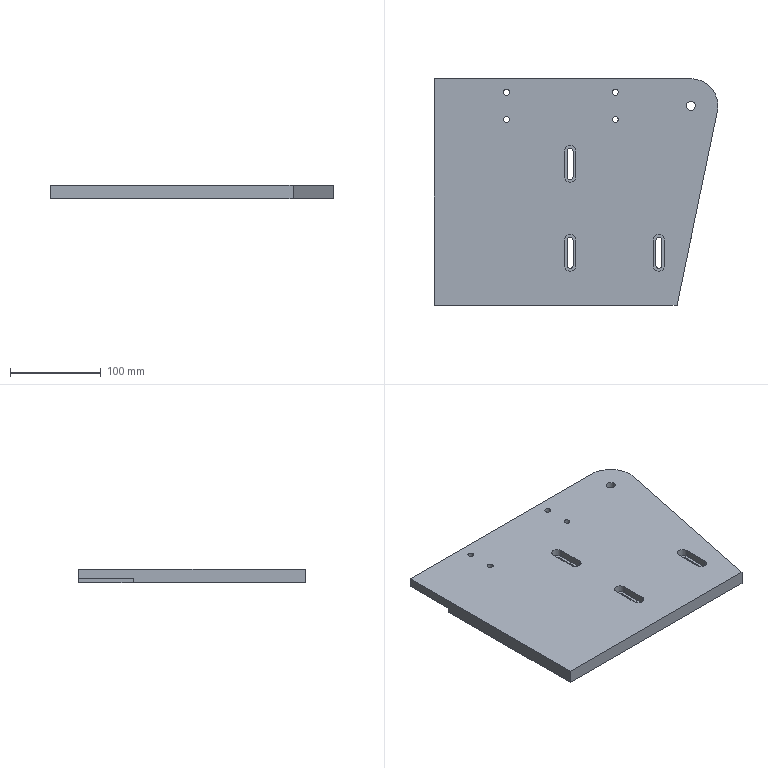Part | NX | 1 solid | 44 faces | box 313.118 x 250 x 15 mm | volume 1008735 mm3 | plane 25 | cylinder 19 | commonest cylinder face diameters 6.5 x10 12.5 x6 10 x1 20 x1 60 x1
STEP:
#1=CARTESIAN_POINT('',(210.,-70.,-7.5));
#2=VERTEX_POINT('',#1);
#3=CARTESIAN_POINT('',(210.,-60.,-7.5));
#4=VERTEX_POINT('',#3);
#5=CARTESIAN_POINT('',(210.,-70.,-7.5));
#6=DIRECTION('',(0.,1.,0.));
#7=VECTOR('',#6,1.);
#8=LINE('',#5,#7);
#9=EDGE_CURVE('',#2,#4,#8,.T.);
#10=ORIENTED_EDGE('',*,*,#9,.F.);
#11=CARTESIAN_POINT('',(230.,-70.,-7.5));
#12=VERTEX_POINT('',#11);
#13=CARTESIAN_POINT('',(220.,-70.,-7.5));
#14=DIRECTION('',(0.,0.,-1.));
#15=DIRECTION('',(1.,0.,0.));
#16=AXIS2_PLACEMENT_3D('',#13,#14,#15);
#17=CIRCLE('',#16,10.);
#18=EDGE_CURVE('',#12,#2,#17,.T.);
#19=ORIENTED_EDGE('',*,*,#18,.F.);
#20=CARTESIAN_POINT('',(230.,0.,-7.5));
#21=VERTEX_POINT('',#20);
#22=CARTESIAN_POINT('',(230.,-70.,-7.5));
#23=DIRECTION('',(0.,1.,0.));
#24=VECTOR('',#23,1.);
#25=LINE('',#22,#24);
#26=EDGE_CURVE('',#12,#21,#25,.T.);
#27=ORIENTED_EDGE('',*,*,#26,.T.);
#28=CARTESIAN_POINT('',(283.118,0.,-7.5));
#29=VERTEX_POINT('',#28);
#30=CARTESIAN_POINT('',(283.118,0.,-7.5));
#31=DIRECTION('',(-1.,0.,0.));
#32=VECTOR('',#31,1.);
#33=LINE('',#30,#32);
#34=EDGE_CURVE('',#29,#21,#33,.T.);
#35=ORIENTED_EDGE('',*,*,#34,.F.);
#36=CARTESIAN_POINT('',(312.489,-36.109,-7.5));
#37=VERTEX_POINT('',#36);
#38=CARTESIAN_POINT('',(283.118,-30.,-7.5));
#39=DIRECTION('',(0.,0.,-1.));
#40=DIRECTION('',(0.,1.,0.));
#41=AXIS2_PLACEMENT_3D('',#38,#39,#40);
#42=CIRCLE('',#41,30.);
#43=EDGE_CURVE('',#29,#37,#42,.T.);
#44=ORIENTED_EDGE('',*,*,#43,.T.);
#45=CARTESIAN_POINT('',(268.,-250.,-7.5));
#46=VERTEX_POINT('',#45);
#47=CARTESIAN_POINT('',(268.,-250.,-7.5));
#48=DIRECTION('',(0.2036,0.979,0.));
#49=VECTOR('',#48,1.);
#50=LINE('',#47,#49);
#51=EDGE_CURVE('',#46,#37,#50,.T.);
#52=ORIENTED_EDGE('',*,*,#51,.F.);
#53=CARTESIAN_POINT('',(0.,-250.,-7.5));
#54=VERTEX_POINT('',#53);
#55=CARTESIAN_POINT('',(0.,-250.,-7.5));
#56=DIRECTION('',(1.,0.,0.));
#57=VECTOR('',#56,1.);
#58=LINE('',#55,#57);
#59=EDGE_CURVE('',#54,#46,#58,.T.);
#60=ORIENTED_EDGE('',*,*,#59,.F.);
#61=CARTESIAN_POINT('',(0.,-60.,-7.5));
#62=VERTEX_POINT('',#61);
#63=CARTESIAN_POINT('',(0.,-60.,-7.5));
#64=DIRECTION('',(0.,-1.,0.));
#65=VECTOR('',#64,1.);
#66=LINE('',#63,#65);
#67=EDGE_CURVE('',#62,#54,#66,.T.);
#68=ORIENTED_EDGE('',*,*,#67,.F.);
#69=CARTESIAN_POINT('',(0.,-60.,-7.5));
#70=DIRECTION('',(1.,0.,0.));
#71=VECTOR('',#70,1.);
#72=LINE('',#69,#71);
#73=EDGE_CURVE('',#62,#4,#72,.T.);
#74=ORIENTED_EDGE('',*,*,#73,.T.);
#75=EDGE_LOOP('',(#10,#19,#27,#35,#44,#52,#60,#68,#74));
#76=FACE_BOUND('',#75,.T.);
#77=CARTESIAN_POINT('',(278.118,-30.,-7.5));
#78=VERTEX_POINT('',#77);
#79=CARTESIAN_POINT('',(283.118,-30.,-7.5));
#80=DIRECTION('',(0.,0.,1.));
#81=DIRECTION('',(1.,0.,0.));
#82=AXIS2_PLACEMENT_3D('',#79,#80,#81);
#83=CIRCLE('',#82,5.);
#84=EDGE_CURVE('',#78,#78,#83,.T.);
#85=ORIENTED_EDGE('',*,*,#84,.T.);
#86=EDGE_LOOP('',(#85));
#87=FACE_BOUND('',#86,.T.);
#88=CARTESIAN_POINT('',(153.25,-80.,-7.5));
#89=VERTEX_POINT('',#88);
#90=CARTESIAN_POINT('',(153.25,-108.,-7.5));
#91=VERTEX_POINT('',#90);
#92=CARTESIAN_POINT('',(153.25,-80.,-7.5));
#93=DIRECTION('',(0.,-1.,0.));
#94=VECTOR('',#93,1.);
#95=LINE('',#92,#94);
#96=EDGE_CURVE('',#89,#91,#95,.T.);
#97=ORIENTED_EDGE('',*,*,#96,.F.);
#98=CARTESIAN_POINT('',(146.75,-80.,-7.5));
#99=VERTEX_POINT('',#98);
#100=CARTESIAN_POINT('',(150.,-80.,-7.5));
#101=DIRECTION('',(0.,0.,-1.));
#102=DIRECTION('',(-1.,0.,0.));
#103=AXIS2_PLACEMENT_3D('',#100,#101,#102);
#104=CIRCLE('',#103,3.25);
#105=EDGE_CURVE('',#99,#89,#104,.T.);
#106=ORIENTED_EDGE('',*,*,#105,.F.);
#107=CARTESIAN_POINT('',(146.75,-108.,-7.5));
#108=VERTEX_POINT('',#107);
#109=CARTESIAN_POINT('',(146.75,-108.,-7.5));
#110=DIRECTION('',(0.,1.,0.));
#111=VECTOR('',#110,1.);
#112=LINE('',#109,#111);
#113=EDGE_CURVE('',#108,#99,#112,.T.);
#114=ORIENTED_EDGE('',*,*,#113,.F.);
#115=CARTESIAN_POINT('',(150.,-108.,-7.5));
#116=DIRECTION('',(0.,0.,-1.));
#117=DIRECTION('',(1.,0.,0.));
#118=AXIS2_PLACEMENT_3D('',#115,#116,#117);
#119=CIRCLE('',#118,3.25);
#120=EDGE_CURVE('',#91,#108,#119,.T.);
#121=ORIENTED_EDGE('',*,*,#120,.F.);
#122=EDGE_LOOP('',(#97,#106,#114,#121));
#123=FACE_BOUND('',#122,.T.);
#124=CARTESIAN_POINT('',(153.25,-178.,-7.5));
#125=VERTEX_POINT('',#124);
#126=CARTESIAN_POINT('',(153.25,-206.,-7.5));
#127=VERTEX_POINT('',#126);
#128=CARTESIAN_POINT('',(153.25,-178.,-7.5));
#129=DIRECTION('',(0.,-1.,0.));
#130=VECTOR('',#129,1.);
#131=LINE('',#128,#130);
#132=EDGE_CURVE('',#125,#127,#131,.T.);
#133=ORIENTED_EDGE('',*,*,#132,.F.);
#134=CARTESIAN_POINT('',(146.75,-178.,-7.5));
#135=VERTEX_POINT('',#134);
#136=CARTESIAN_POINT('',(150.,-178.,-7.5));
#137=DIRECTION('',(0.,0.,-1.));
#138=DIRECTION('',(-1.,0.,0.));
#139=AXIS2_PLACEMENT_3D('',#136,#137,#138);
#140=CIRCLE('',#139,3.25);
#141=EDGE_CURVE('',#135,#125,#140,.T.);
#142=ORIENTED_EDGE('',*,*,#141,.F.);
#143=CARTESIAN_POINT('',(146.75,-206.,-7.5));
#144=VERTEX_POINT('',#143);
#145=CARTESIAN_POINT('',(146.75,-206.,-7.5));
#146=DIRECTION('',(0.,1.,0.));
#147=VECTOR('',#146,1.);
#148=LINE('',#145,#147);
#149=EDGE_CURVE('',#144,#135,#148,.T.);
#150=ORIENTED_EDGE('',*,*,#149,.F.);
#151=CARTESIAN_POINT('',(150.,-206.,-7.5));
#152=DIRECTION('',(0.,0.,-1.));
#153=DIRECTION('',(1.,0.,0.));
#154=AXIS2_PLACEMENT_3D('',#151,#152,#153);
#155=CIRCLE('',#154,3.25);
#156=EDGE_CURVE('',#127,#144,#155,.T.);
#157=ORIENTED_EDGE('',*,*,#156,.F.);
#158=EDGE_LOOP('',(#133,#142,#150,#157));
#159=FACE_BOUND('',#158,.T.);
#160=CARTESIAN_POINT('',(251.25,-178.,-7.5));
#161=VERTEX_POINT('',#160);
#162=CARTESIAN_POINT('',(251.25,-206.,-7.5));
#163=VERTEX_POINT('',#162);
#164=CARTESIAN_POINT('',(251.25,-178.,-7.5));
#165=DIRECTION('',(0.,-1.,0.));
#166=VECTOR('',#165,1.);
#167=LINE('',#164,#166);
#168=EDGE_CURVE('',#161,#163,#167,.T.);
#169=ORIENTED_EDGE('',*,*,#168,.F.);
#170=CARTESIAN_POINT('',(244.75,-178.,-7.5));
#171=VERTEX_POINT('',#170);
#172=CARTESIAN_POINT('',(248.,-178.,-7.5));
#173=DIRECTION('',(0.,0.,-1.));
#174=DIRECTION('',(-1.,0.,0.));
#175=AXIS2_PLACEMENT_3D('',#172,#173,#174);
#176=CIRCLE('',#175,3.25);
#177=EDGE_CURVE('',#171,#161,#176,.T.);
#178=ORIENTED_EDGE('',*,*,#177,.F.);
#179=CARTESIAN_POINT('',(244.75,-206.,-7.5));
#180=VERTEX_POINT('',#179);
#181=CARTESIAN_POINT('',(244.75,-206.,-7.5));
#182=DIRECTION('',(0.,1.,0.));
#183=VECTOR('',#182,1.);
#184=LINE('',#181,#183);
#185=EDGE_CURVE('',#180,#171,#184,.T.);
#186=ORIENTED_EDGE('',*,*,#185,.F.);
#187=CARTESIAN_POINT('',(248.,-206.,-7.5));
#188=DIRECTION('',(0.,0.,-1.));
#189=DIRECTION('',(1.,0.,0.));
#190=AXIS2_PLACEMENT_3D('',#187,#188,#189);
#191=CIRCLE('',#190,3.25);
#192=EDGE_CURVE('',#163,#180,#191,.T.);
#193=ORIENTED_EDGE('',*,*,#192,.F.);
#194=EDGE_LOOP('',(#169,#178,#186,#193));
#195=FACE_BOUND('',#194,.T.);
#196=CARTESIAN_POINT('',(0.,0.,-7.5));
#197=DIRECTION('',(0.,0.,1.));
#198=DIRECTION('',(1.,0.,0.));
#199=AXIS2_PLACEMENT_3D('',#196,#197,#198);
#200=PLANE('',#199);
#201=ADVANCED_FACE('',(#76,#87,#123,#159,#195),#200,.F.);
#202=CARTESIAN_POINT('',(312.489,-36.109,7.5));
#203=VERTEX_POINT('',#202);
#204=CARTESIAN_POINT('',(283.118,0.,7.5));
#205=VERTEX_POINT('',#204);
#206=CARTESIAN_POINT('',(283.118,-30.,7.5));
#207=DIRECTION('',(0.,0.,1.));
#208=DIRECTION('',(0.979,-0.2036,0.));
#209=AXIS2_PLACEMENT_3D('',#206,#207,#208);
#210=CIRCLE('',#209,30.);
#211=EDGE_CURVE('',#203,#205,#210,.T.);
#212=ORIENTED_EDGE('',*,*,#211,.T.);
#213=CARTESIAN_POINT('',(0.,0.,7.5));
#214=VERTEX_POINT('',#213);
#215=CARTESIAN_POINT('',(283.118,0.,7.5));
#216=DIRECTION('',(-1.,0.,0.));
#217=VECTOR('',#216,1.);
#218=LINE('',#215,#217);
#219=EDGE_CURVE('',#205,#214,#218,.T.);
#220=ORIENTED_EDGE('',*,*,#219,.T.);
#221=CARTESIAN_POINT('',(0.,-250.,7.5));
#222=VERTEX_POINT('',#221);
#223=CARTESIAN_POINT('',(0.,0.,7.5));
#224=DIRECTION('',(0.,-1.,0.));
#225=VECTOR('',#224,1.);
#226=LINE('',#223,#225);
#227=EDGE_CURVE('',#214,#222,#226,.T.);
#228=ORIENTED_EDGE('',*,*,#227,.T.);
#229=CARTESIAN_POINT('',(268.,-250.,7.5));
#230=VERTEX_POINT('',#229);
#231=CARTESIAN_POINT('',(0.,-250.,7.5));
#232=DIRECTION('',(1.,0.,0.));
#233=VECTOR('',#232,1.);
#234=LINE('',#231,#233);
#235=EDGE_CURVE('',#222,#230,#234,.T.);
#236=ORIENTED_EDGE('',*,*,#235,.T.);
#237=CARTESIAN_POINT('',(268.,-250.,7.5));
#238=DIRECTION('',(0.2036,0.979,0.));
#239=VECTOR('',#238,1.);
#240=LINE('',#237,#239);
#241=EDGE_CURVE('',#230,#203,#240,.T.);
#242=ORIENTED_EDGE('',*,*,#241,.T.);
#243=EDGE_LOOP('',(#212,#220,#228,#236,#242));
#244=FACE_BOUND('',#243,.T.);
#245=CARTESIAN_POINT('',(278.118,-30.,7.5));
#246=VERTEX_POINT('',#245);
#247=CARTESIAN_POINT('',(283.118,-30.,7.5));
#248=DIRECTION('',(0.,0.,1.));
#249=DIRECTION('',(1.,0.,0.));
#250=AXIS2_PLACEMENT_3D('',#247,#248,#249);
#251=CIRCLE('',#250,5.);
#252=EDGE_CURVE('',#246,#246,#251,.T.);
#253=ORIENTED_EDGE('',*,*,#252,.F.);
#254=EDGE_LOOP('',(#253));
#255=FACE_BOUND('',#254,.T.);
#256=CARTESIAN_POINT('',(254.25,-178.,7.5));
#257=VERTEX_POINT('',#256);
#258=CARTESIAN_POINT('',(241.75,-178.,7.5));
#259=VERTEX_POINT('',#258);
#260=CARTESIAN_POINT('',(248.,-178.,7.5));
#261=DIRECTION('',(0.,0.,1.));
#262=DIRECTION('',(1.,0.,0.));
#263=AXIS2_PLACEMENT_3D('',#260,#261,#262);
#264=CIRCLE('',#263,6.25);
#265=EDGE_CURVE('',#257,#259,#264,.T.);
#266=ORIENTED_EDGE('',*,*,#265,.F.);
#267=CARTESIAN_POINT('',(254.25,-206.,7.5));
#268=VERTEX_POINT('',#267);
#269=CARTESIAN_POINT('',(254.25,-206.,7.5));
#270=DIRECTION('',(0.,1.,0.));
#271=VECTOR('',#270,1.);
#272=LINE('',#269,#271);
#273=EDGE_CURVE('',#268,#257,#272,.T.);
#274=ORIENTED_EDGE('',*,*,#273,.F.);
#275=CARTESIAN_POINT('',(241.75,-206.,7.5));
#276=VERTEX_POINT('',#275);
#277=CARTESIAN_POINT('',(248.,-206.,7.5));
#278=DIRECTION('',(0.,0.,1.));
#279=DIRECTION('',(-1.,0.,0.));
#280=AXIS2_PLACEMENT_3D('',#277,#278,#279);
#281=CIRCLE('',#280,6.25);
#282=EDGE_CURVE('',#276,#268,#281,.T.);
#283=ORIENTED_EDGE('',*,*,#282,.F.);
#284=CARTESIAN_POINT('',(241.75,-178.,7.5));
#285=DIRECTION('',(0.,-1.,0.));
#286=VECTOR('',#285,1.);
#287=LINE('',#284,#286);
#288=EDGE_CURVE('',#259,#276,#287,.T.);
#289=ORIENTED_EDGE('',*,*,#288,.F.);
#290=EDGE_LOOP('',(#266,#274,#283,#289));
#291=FACE_BOUND('',#290,.T.);
#292=CARTESIAN_POINT('',(156.25,-178.,7.5));
#293=VERTEX_POINT('',#292);
#294=CARTESIAN_POINT('',(143.75,-178.,7.5));
#295=VERTEX_POINT('',#294);
#296=CARTESIAN_POINT('',(150.,-178.,7.5));
#297=DIRECTION('',(0.,0.,1.));
#298=DIRECTION('',(1.,0.,0.));
#299=AXIS2_PLACEMENT_3D('',#296,#297,#298);
#300=CIRCLE('',#299,6.25);
#301=EDGE_CURVE('',#293,#295,#300,.T.);
#302=ORIENTED_EDGE('',*,*,#301,.F.);
#303=CARTESIAN_POINT('',(156.25,-206.,7.5));
#304=VERTEX_POINT('',#303);
#305=CARTESIAN_POINT('',(156.25,-206.,7.5));
#306=DIRECTION('',(0.,1.,0.));
#307=VECTOR('',#306,1.);
#308=LINE('',#305,#307);
#309=EDGE_CURVE('',#304,#293,#308,.T.);
#310=ORIENTED_EDGE('',*,*,#309,.F.);
#311=CARTESIAN_POINT('',(143.75,-206.,7.5));
#312=VERTEX_POINT('',#311);
#313=CARTESIAN_POINT('',(150.,-206.,7.5));
#314=DIRECTION('',(0.,0.,1.));
#315=DIRECTION('',(-1.,0.,0.));
#316=AXIS2_PLACEMENT_3D('',#313,#314,#315);
#317=CIRCLE('',#316,6.25);
#318=EDGE_CURVE('',#312,#304,#317,.T.);
#319=ORIENTED_EDGE('',*,*,#318,.F.);
#320=CARTESIAN_POINT('',(143.75,-178.,7.5));
#321=DIRECTION('',(0.,-1.,0.));
#322=VECTOR('',#321,1.);
#323=LINE('',#320,#322);
#324=EDGE_CURVE('',#295,#312,#323,.T.);
#325=ORIENTED_EDGE('',*,*,#324,.F.);
#326=EDGE_LOOP('',(#302,#310,#319,#325));
#327=FACE_BOUND('',#326,.T.);
#328=CARTESIAN_POINT('',(156.25,-80.,7.5));
#329=VERTEX_POINT('',#328);
#330=CARTESIAN_POINT('',(143.75,-80.,7.5));
#331=VERTEX_POINT('',#330);
#332=CARTESIAN_POINT('',(150.,-80.,7.5));
#333=DIRECTION('',(0.,0.,1.));
#334=DIRECTION('',(1.,0.,0.));
#335=AXIS2_PLACEMENT_3D('',#332,#333,#334);
#336=CIRCLE('',#335,6.25);
#337=EDGE_CURVE('',#329,#331,#336,.T.);
#338=ORIENTED_EDGE('',*,*,#337,.F.);
#339=CARTESIAN_POINT('',(156.25,-108.,7.5));
#340=VERTEX_POINT('',#339);
#341=CARTESIAN_POINT('',(156.25,-108.,7.5));
#342=DIRECTION('',(0.,1.,0.));
#343=VECTOR('',#342,1.);
#344=LINE('',#341,#343);
#345=EDGE_CURVE('',#340,#329,#344,.T.);
#346=ORIENTED_EDGE('',*,*,#345,.F.);
#347=CARTESIAN_POINT('',(143.75,-108.,7.5));
#348=VERTEX_POINT('',#347);
#349=CARTESIAN_POINT('',(150.,-108.,7.5));
#350=DIRECTION('',(0.,0.,1.));
#351=DIRECTION('',(-1.,0.,0.));
#352=AXIS2_PLACEMENT_3D('',#349,#350,#351);
#353=CIRCLE('',#352,6.25);
#354=EDGE_CURVE('',#348,#340,#353,.T.);
#355=ORIENTED_EDGE('',*,*,#354,.F.);
#356=CARTESIAN_POINT('',(143.75,-80.,7.5));
#357=DIRECTION('',(0.,-1.,0.));
#358=VECTOR('',#357,1.);
#359=LINE('',#356,#358);
#360=EDGE_CURVE('',#331,#348,#359,.T.);
#361=ORIENTED_EDGE('',*,*,#360,.F.);
#362=EDGE_LOOP('',(#338,#346,#355,#361));
#363=FACE_BOUND('',#362,.T.);
#364=CARTESIAN_POINT('',(83.25,-15.,7.5));
#365=VERTEX_POINT('',#364);
#366=CARTESIAN_POINT('',(80.,-15.,7.5));
#367=DIRECTION('',(0.,0.,1.));
#368=DIRECTION('',(1.,0.,0.));
#369=AXIS2_PLACEMENT_3D('',#366,#367,#368);
#370=CIRCLE('',#369,3.25);
#371=EDGE_CURVE('',#365,#365,#370,.T.);
#372=ORIENTED_EDGE('',*,*,#371,.F.);
#373=EDGE_LOOP('',(#372));
#374=FACE_BOUND('',#373,.T.);
#375=CARTESIAN_POINT('',(83.25,-45.,7.5));
#376=VERTEX_POINT('',#375);
#377=CARTESIAN_POINT('',(80.,-45.,7.5));
#378=DIRECTION('',(0.,0.,1.));
#379=DIRECTION('',(1.,0.,0.));
#380=AXIS2_PLACEMENT_3D('',#377,#378,#379);
#381=CIRCLE('',#380,3.25);
#382=EDGE_CURVE('',#376,#376,#381,.T.);
#383=ORIENTED_EDGE('',*,*,#382,.F.);
#384=EDGE_LOOP('',(#383));
#385=FACE_BOUND('',#384,.T.);
#386=CARTESIAN_POINT('',(203.25,-15.,7.5));
#387=VERTEX_POINT('',#386);
#388=CARTESIAN_POINT('',(200.,-15.,7.5));
#389=DIRECTION('',(0.,0.,1.));
#390=DIRECTION('',(1.,0.,0.));
#391=AXIS2_PLACEMENT_3D('',#388,#389,#390);
#392=CIRCLE('',#391,3.25);
#393=EDGE_CURVE('',#387,#387,#392,.T.);
#394=ORIENTED_EDGE('',*,*,#393,.F.);
#395=EDGE_LOOP('',(#394));
#396=FACE_BOUND('',#395,.T.);
#397=CARTESIAN_POINT('',(203.25,-45.,7.5));
#398=VERTEX_POINT('',#397);
#399=CARTESIAN_POINT('',(200.,-45.,7.5));
#400=DIRECTION('',(0.,0.,1.));
#401=DIRECTION('',(1.,0.,0.));
#402=AXIS2_PLACEMENT_3D('',#399,#400,#401);
#403=CIRCLE('',#402,3.25);
#404=EDGE_CURVE('',#398,#398,#403,.T.);
#405=ORIENTED_EDGE('',*,*,#404,.F.);
#406=EDGE_LOOP('',(#405));
#407=FACE_BOUND('',#406,.T.);
#408=CARTESIAN_POINT('',(0.,0.,7.5));
#409=DIRECTION('',(0.,0.,1.));
#410=DIRECTION('',(1.,0.,0.));
#411=AXIS2_PLACEMENT_3D('',#408,#409,#410);
#412=PLANE('',#411);
#413=ADVANCED_FACE('',(#244,#255,#291,#327,#363,#374,#385,#396,#407),#412,.T.);
#414=CARTESIAN_POINT('',(0.,0.,-2.5));
#415=VERTEX_POINT('',#414);
#416=CARTESIAN_POINT('',(0.,-60.,-2.5));
#417=VERTEX_POINT('',#416);
#418=CARTESIAN_POINT('',(0.,0.,-2.5));
#419=DIRECTION('',(0.,-1.,0.));
#420=VECTOR('',#419,1.);
#421=LINE('',#418,#420);
#422=EDGE_CURVE('',#415,#417,#421,.T.);
#423=ORIENTED_EDGE('',*,*,#422,.T.);
#424=CARTESIAN_POINT('',(0.,-60.,-7.5));
#425=DIRECTION('',(0.,0.,1.));
#426=VECTOR('',#425,1.);
#427=LINE('',#424,#426);
#428=EDGE_CURVE('',#62,#417,#427,.T.);
#429=ORIENTED_EDGE('',*,*,#428,.F.);
#430=ORIENTED_EDGE('',*,*,#67,.T.);
#431=CARTESIAN_POINT('',(0.,-250.,-7.5));
#432=DIRECTION('',(0.,0.,1.));
#433=VECTOR('',#432,1.);
#434=LINE('',#431,#433);
#435=EDGE_CURVE('',#54,#222,#434,.T.);
#436=ORIENTED_EDGE('',*,*,#435,.T.);
#437=ORIENTED_EDGE('',*,*,#227,.F.);
#438=CARTESIAN_POINT('',(0.,0.,-2.5));
#439=DIRECTION('',(0.,0.,1.));
#440=VECTOR('',#439,1.);
#441=LINE('',#438,#440);
#442=EDGE_CURVE('',#415,#214,#441,.T.);
#443=ORIENTED_EDGE('',*,*,#442,.F.);
#444=EDGE_LOOP('',(#423,#429,#430,#436,#437,#443));
#445=FACE_OUTER_BOUND('',#444,.T.);
#446=CARTESIAN_POINT('',(0.,0.,-7.5));
#447=DIRECTION('',(-1.,0.,0.));
#448=DIRECTION('',(0.,0.,1.));
#449=AXIS2_PLACEMENT_3D('',#446,#447,#448);
#450=PLANE('',#449);
#451=ADVANCED_FACE('',(#445),#450,.T.);
#452=ORIENTED_EDGE('',*,*,#59,.T.);
#453=CARTESIAN_POINT('',(268.,-250.,-7.5));
#454=DIRECTION('',(0.,0.,1.));
#455=VECTOR('',#454,1.);
#456=LINE('',#453,#455);
#457=EDGE_CURVE('',#46,#230,#456,.T.);
#458=ORIENTED_EDGE('',*,*,#457,.T.);
#459=ORIENTED_EDGE('',*,*,#235,.F.);
#460=ORIENTED_EDGE('',*,*,#435,.F.);
#461=EDGE_LOOP('',(#452,#458,#459,#460));
#462=FACE_OUTER_BOUND('',#461,.T.);
#463=CARTESIAN_POINT('',(0.,-250.,-7.5));
#464=DIRECTION('',(0.,-1.,0.));
#465=DIRECTION('',(0.,0.,-1.));
#466=AXIS2_PLACEMENT_3D('',#463,#464,#465);
#467=PLANE('',#466);
#468=ADVANCED_FACE('',(#462),#467,.T.);
#469=CARTESIAN_POINT('',(312.489,-36.109,7.5));
#470=DIRECTION('',(0.,0.,-1.));
#471=VECTOR('',#470,1.);
#472=LINE('',#469,#471);
#473=EDGE_CURVE('',#203,#37,#472,.T.);
#474=ORIENTED_EDGE('',*,*,#473,.F.);
#475=ORIENTED_EDGE('',*,*,#241,.F.);
#476=ORIENTED_EDGE('',*,*,#457,.F.);
#477=ORIENTED_EDGE('',*,*,#51,.T.);
#478=EDGE_LOOP('',(#474,#475,#476,#477));
#479=FACE_OUTER_BOUND('',#478,.T.);
#480=CARTESIAN_POINT('',(268.,-250.,-7.5));
#481=DIRECTION('',(0.979,-0.2036,0.));
#482=DIRECTION('',(0.,0.,-1.));
#483=AXIS2_PLACEMENT_3D('',#480,#481,#482);
#484=PLANE('',#483);
#485=ADVANCED_FACE('',(#479),#484,.T.);
#486=CARTESIAN_POINT('',(230.,0.,-2.5));
#487=VERTEX_POINT('',#486);
#488=CARTESIAN_POINT('',(0.,0.,-2.5));
#489=DIRECTION('',(1.,0.,0.));
#490=VECTOR('',#489,1.);
#491=LINE('',#488,#490);
#492=EDGE_CURVE('',#415,#487,#491,.T.);
#493=ORIENTED_EDGE('',*,*,#492,.F.);
#494=ORIENTED_EDGE('',*,*,#442,.T.);
#495=ORIENTED_EDGE('',*,*,#219,.F.);
#496=CARTESIAN_POINT('',(283.118,0.,7.5));
#497=DIRECTION('',(0.,0.,-1.));
#498=VECTOR('',#497,1.);
#499=LINE('',#496,#498);
#500=EDGE_CURVE('',#205,#29,#499,.T.);
#501=ORIENTED_EDGE('',*,*,#500,.T.);
#502=ORIENTED_EDGE('',*,*,#34,.T.);
#503=CARTESIAN_POINT('',(230.,0.,-7.5));
#504=DIRECTION('',(0.,0.,1.));
#505=VECTOR('',#504,1.);
#506=LINE('',#503,#505);
#507=EDGE_CURVE('',#21,#487,#506,.T.);
#508=ORIENTED_EDGE('',*,*,#507,.T.);
#509=EDGE_LOOP('',(#493,#494,#495,#501,#502,#508));
#510=FACE_OUTER_BOUND('',#509,.T.);
#511=CARTESIAN_POINT('',(320.,0.,-7.5));
#512=DIRECTION('',(0.,1.,0.));
#513=DIRECTION('',(0.,0.,1.));
#514=AXIS2_PLACEMENT_3D('',#511,#512,#513);
#515=PLANE('',#514);
#516=ADVANCED_FACE('',(#510),#515,.T.);
#517=ORIENTED_EDGE('',*,*,#43,.F.);
#518=ORIENTED_EDGE('',*,*,#500,.F.);
#519=ORIENTED_EDGE('',*,*,#211,.F.);
#520=ORIENTED_EDGE('',*,*,#473,.T.);
#521=EDGE_LOOP('',(#517,#518,#519,#520));
#522=FACE_OUTER_BOUND('',#521,.T.);
#523=CARTESIAN_POINT('',(283.118,-30.,8.136));
#524=DIRECTION('',(0.,0.,-1.));
#525=DIRECTION('',(0.,1.,0.));
#526=AXIS2_PLACEMENT_3D('',#523,#524,#525);
#527=CYLINDRICAL_SURFACE('',#526,30.);
#528=ADVANCED_FACE('',(#522),#527,.T.);
#529=CARTESIAN_POINT('',(210.,-60.,-2.5));
#530=VERTEX_POINT('',#529);
#531=CARTESIAN_POINT('',(210.,-60.,-2.5));
#532=DIRECTION('',(-1.,0.,0.));
#533=VECTOR('',#532,1.);
#534=LINE('',#531,#533);
#535=EDGE_CURVE('',#530,#417,#534,.T.);
#536=ORIENTED_EDGE('',*,*,#535,.T.);
#537=ORIENTED_EDGE('',*,*,#422,.F.);
#538=ORIENTED_EDGE('',*,*,#492,.T.);
#539=CARTESIAN_POINT('',(230.,-70.,-2.5));
#540=VERTEX_POINT('',#539);
#541=CARTESIAN_POINT('',(230.,-70.,-2.5));
#542=DIRECTION('',(0.,1.,0.));
#543=VECTOR('',#542,1.);
#544=LINE('',#541,#543);
#545=EDGE_CURVE('',#540,#487,#544,.T.);
#546=ORIENTED_EDGE('',*,*,#545,.F.);
#547=CARTESIAN_POINT('',(210.,-70.,-2.5));
#548=VERTEX_POINT('',#547);
#549=CARTESIAN_POINT('',(220.,-70.,-2.5));
#550=DIRECTION('',(0.,0.,-1.));
#551=DIRECTION('',(1.,0.,0.));
#552=AXIS2_PLACEMENT_3D('',#549,#550,#551);
#553=CIRCLE('',#552,10.);
#554=EDGE_CURVE('',#540,#548,#553,.T.);
#555=ORIENTED_EDGE('',*,*,#554,.T.);
#556=CARTESIAN_POINT('',(210.,-70.,-2.5));
#557=DIRECTION('',(0.,1.,0.));
#558=VECTOR('',#557,1.);
#559=LINE('',#556,#558);
#560=EDGE_CURVE('',#548,#530,#559,.T.);
#561=ORIENTED_EDGE('',*,*,#560,.T.);
#562=EDGE_LOOP('',(#536,#537,#538,#546,#555,#561));
#563=FACE_BOUND('',#562,.T.);
#564=CARTESIAN_POINT('',(83.25,-15.,-2.5));
#565=VERTEX_POINT('',#564);
#566=CARTESIAN_POINT('',(80.,-15.,-2.5));
#567=DIRECTION('',(0.,0.,1.));
#568=DIRECTION('',(1.,0.,0.));
#569=AXIS2_PLACEMENT_3D('',#566,#567,#568);
#570=CIRCLE('',#569,3.25);
#571=EDGE_CURVE('',#565,#565,#570,.T.);
#572=ORIENTED_EDGE('',*,*,#571,.T.);
#573=EDGE_LOOP('',(#572));
#574=FACE_BOUND('',#573,.T.);
#575=CARTESIAN_POINT('',(83.25,-45.,-2.5));
#576=VERTEX_POINT('',#575);
#577=CARTESIAN_POINT('',(80.,-45.,-2.5));
#578=DIRECTION('',(0.,0.,1.));
#579=DIRECTION('',(1.,0.,0.));
#580=AXIS2_PLACEMENT_3D('',#577,#578,#579);
#581=CIRCLE('',#580,3.25);
#582=EDGE_CURVE('',#576,#576,#581,.T.);
#583=ORIENTED_EDGE('',*,*,#582,.T.);
#584=EDGE_LOOP('',(#583));
#585=FACE_BOUND('',#584,.T.);
#586=CARTESIAN_POINT('',(203.25,-15.,-2.5));
#587=VERTEX_POINT('',#586);
#588=CARTESIAN_POINT('',(200.,-15.,-2.5));
#589=DIRECTION('',(0.,0.,1.));
#590=DIRECTION('',(1.,0.,0.));
#591=AXIS2_PLACEMENT_3D('',#588,#589,#590);
#592=CIRCLE('',#591,3.25);
#593=EDGE_CURVE('',#587,#587,#592,.T.);
#594=ORIENTED_EDGE('',*,*,#593,.T.);
#595=EDGE_LOOP('',(#594));
#596=FACE_BOUND('',#595,.T.);
#597=CARTESIAN_POINT('',(203.25,-45.,-2.5));
#598=VERTEX_POINT('',#597);
#599=CARTESIAN_POINT('',(200.,-45.,-2.5));
#600=DIRECTION('',(0.,0.,1.));
#601=DIRECTION('',(1.,0.,0.));
#602=AXIS2_PLACEMENT_3D('',#599,#600,#601);
#603=CIRCLE('',#602,3.25);
#604=EDGE_CURVE('',#598,#598,#603,.T.);
#605=ORIENTED_EDGE('',*,*,#604,.T.);
#606=EDGE_LOOP('',(#605));
#607=FACE_BOUND('',#606,.T.);
#608=CARTESIAN_POINT('',(0.,0.,-2.5));
#609=DIRECTION('',(0.,0.,-1.));
#610=DIRECTION('',(-1.,0.,0.));
#611=AXIS2_PLACEMENT_3D('',#608,#609,#610);
#612=PLANE('',#611);
#613=ADVANCED_FACE('',(#563,#574,#585,#596,#607),#612,.T.);
#614=ORIENTED_EDGE('',*,*,#545,.T.);
#615=ORIENTED_EDGE('',*,*,#507,.F.);
#616=ORIENTED_EDGE('',*,*,#26,.F.);
#617=CARTESIAN_POINT('',(230.,-70.,-7.5));
#618=DIRECTION('',(0.,0.,1.));
#619=VECTOR('',#618,1.);
#620=LINE('',#617,#619);
#621=EDGE_CURVE('',#12,#540,#620,.T.);
#622=ORIENTED_EDGE('',*,*,#621,.T.);
#623=EDGE_LOOP('',(#614,#615,#616,#622));
#624=FACE_OUTER_BOUND('',#623,.T.);
#625=CARTESIAN_POINT('',(230.,0.,-7.5));
#626=DIRECTION('',(1.,0.,0.));
#627=DIRECTION('',(0.,0.,-1.));
#628=AXIS2_PLACEMENT_3D('',#625,#626,#627);
#629=PLANE('',#628);
#630=ADVANCED_FACE('',(#624),#629,.F.);
#631=CARTESIAN_POINT('',(210.,-60.,-2.5));
#632=DIRECTION('',(0.,0.,-1.));
#633=VECTOR('',#632,1.);
#634=LINE('',#631,#633);
#635=EDGE_CURVE('',#530,#4,#634,.T.);
#636=ORIENTED_EDGE('',*,*,#635,.T.);
#637=ORIENTED_EDGE('',*,*,#73,.F.);
#638=ORIENTED_EDGE('',*,*,#428,.T.);
#639=ORIENTED_EDGE('',*,*,#535,.F.);
#640=EDGE_LOOP('',(#636,#637,#638,#639));
#641=FACE_OUTER_BOUND('',#640,.T.);
#642=CARTESIAN_POINT('',(230.,-60.,-7.5));
#643=DIRECTION('',(0.,-1.,0.));
#644=DIRECTION('',(0.,0.,-1.));
#645=AXIS2_PLACEMENT_3D('',#642,#643,#644);
#646=PLANE('',#645);
#647=ADVANCED_FACE('',(#641),#646,.F.);
#648=ORIENTED_EDGE('',*,*,#9,.T.);
#649=ORIENTED_EDGE('',*,*,#635,.F.);
#650=ORIENTED_EDGE('',*,*,#560,.F.);
#651=CARTESIAN_POINT('',(210.,-70.,-7.5));
#652=DIRECTION('',(0.,0.,1.));
#653=VECTOR('',#652,1.);
#654=LINE('',#651,#653);
#655=EDGE_CURVE('',#2,#548,#654,.T.);
#656=ORIENTED_EDGE('',*,*,#655,.F.);
#657=EDGE_LOOP('',(#648,#649,#650,#656));
#658=FACE_OUTER_BOUND('',#657,.T.);
#659=CARTESIAN_POINT('',(210.,-70.,-7.5));
#660=DIRECTION('',(-1.,0.,0.));
#661=DIRECTION('',(0.,0.,1.));
#662=AXIS2_PLACEMENT_3D('',#659,#660,#661);
#663=PLANE('',#662);
#664=ADVANCED_FACE('',(#658),#663,.F.);
#665=ORIENTED_EDGE('',*,*,#18,.T.);
#666=ORIENTED_EDGE('',*,*,#655,.T.);
#667=ORIENTED_EDGE('',*,*,#554,.F.);
#668=ORIENTED_EDGE('',*,*,#621,.F.);
#669=EDGE_LOOP('',(#665,#666,#667,#668));
#670=FACE_OUTER_BOUND('',#669,.T.);
#671=CARTESIAN_POINT('',(220.,-70.,-7.5));
#672=DIRECTION('',(0.,0.,-1.));
#673=DIRECTION('',(1.,0.,0.));
#674=AXIS2_PLACEMENT_3D('',#671,#672,#673);
#675=CYLINDRICAL_SURFACE('',#674,10.);
#676=ADVANCED_FACE('',(#670),#675,.F.);
#677=ORIENTED_EDGE('',*,*,#84,.F.);
#678=EDGE_LOOP('',(#677));
#679=FACE_BOUND('',#678,.T.);
#680=ORIENTED_EDGE('',*,*,#252,.T.);
#681=EDGE_LOOP('',(#680));
#682=FACE_BOUND('',#681,.T.);
#683=CARTESIAN_POINT('',(283.118,-30.,7.5));
#684=DIRECTION('',(0.,0.,1.));
#685=DIRECTION('',(1.,0.,0.));
#686=AXIS2_PLACEMENT_3D('',#683,#684,#685);
#687=CYLINDRICAL_SURFACE('',#686,5.);
#688=ADVANCED_FACE('',(#679,#682),#687,.F.);
#689=CARTESIAN_POINT('',(153.25,-80.,-0.5));
#690=VERTEX_POINT('',#689);
#691=CARTESIAN_POINT('',(153.25,-108.,-0.5));
#692=VERTEX_POINT('',#691);
#693=CARTESIAN_POINT('',(153.25,-80.,-0.5));
#694=DIRECTION('',(0.,-1.,0.));
#695=VECTOR('',#694,1.);
#696=LINE('',#693,#695);
#697=EDGE_CURVE('',#690,#692,#696,.T.);
#698=ORIENTED_EDGE('',*,*,#697,.F.);
#699=CARTESIAN_POINT('',(153.25,-80.,-7.5));
#700=DIRECTION('',(0.,0.,1.));
#701=VECTOR('',#700,1.);
#702=LINE('',#699,#701);
#703=EDGE_CURVE('',#89,#690,#702,.T.);
#704=ORIENTED_EDGE('',*,*,#703,.F.);
#705=ORIENTED_EDGE('',*,*,#96,.T.);
#706=CARTESIAN_POINT('',(153.25,-108.,-7.5));
#707=DIRECTION('',(0.,0.,1.));
#708=VECTOR('',#707,1.);
#709=LINE('',#706,#708);
#710=EDGE_CURVE('',#91,#692,#709,.T.);
#711=ORIENTED_EDGE('',*,*,#710,.T.);
#712=EDGE_LOOP('',(#698,#704,#705,#711));
#713=FACE_OUTER_BOUND('',#712,.T.);
#714=CARTESIAN_POINT('',(153.25,-80.,-7.5));
#715=DIRECTION('',(1.,0.,0.));
#716=DIRECTION('',(0.,0.,-1.));
#717=AXIS2_PLACEMENT_3D('',#714,#715,#716);
#718=PLANE('',#717);
#719=ADVANCED_FACE('',(#713),#718,.F.);
#720=CARTESIAN_POINT('',(146.75,-108.,-0.5));
#721=VERTEX_POINT('',#720);
#722=CARTESIAN_POINT('',(150.,-108.,-0.5));
#723=DIRECTION('',(0.,0.,-1.));
#724=DIRECTION('',(1.,0.,0.));
#725=AXIS2_PLACEMENT_3D('',#722,#723,#724);
#726=CIRCLE('',#725,3.25);
#727=EDGE_CURVE('',#692,#721,#726,.T.);
#728=ORIENTED_EDGE('',*,*,#727,.F.);
#729=ORIENTED_EDGE('',*,*,#710,.F.);
#730=ORIENTED_EDGE('',*,*,#120,.T.);
#731=CARTESIAN_POINT('',(146.75,-108.,-7.5));
#732=DIRECTION('',(0.,0.,1.));
#733=VECTOR('',#732,1.);
#734=LINE('',#731,#733);
#735=EDGE_CURVE('',#108,#721,#734,.T.);
#736=ORIENTED_EDGE('',*,*,#735,.T.);
#737=EDGE_LOOP('',(#728,#729,#730,#736));
#738=FACE_OUTER_BOUND('',#737,.T.);
#739=CARTESIAN_POINT('',(150.,-108.,-7.5));
#740=DIRECTION('',(0.,0.,-1.));
#741=DIRECTION('',(-1.,0.,0.));
#742=AXIS2_PLACEMENT_3D('',#739,#740,#741);
#743=CYLINDRICAL_SURFACE('',#742,3.25);
#744=ADVANCED_FACE('',(#738),#743,.F.);
#745=CARTESIAN_POINT('',(146.75,-80.,-0.5));
#746=VERTEX_POINT('',#745);
#747=CARTESIAN_POINT('',(146.75,-108.,-0.5));
#748=DIRECTION('',(0.,1.,0.));
#749=VECTOR('',#748,1.);
#750=LINE('',#747,#749);
#751=EDGE_CURVE('',#721,#746,#750,.T.);
#752=ORIENTED_EDGE('',*,*,#751,.F.);
#753=ORIENTED_EDGE('',*,*,#735,.F.);
#754=ORIENTED_EDGE('',*,*,#113,.T.);
#755=CARTESIAN_POINT('',(146.75,-80.,-7.5));
#756=DIRECTION('',(0.,0.,1.));
#757=VECTOR('',#756,1.);
#758=LINE('',#755,#757);
#759=EDGE_CURVE('',#99,#746,#758,.T.);
#760=ORIENTED_EDGE('',*,*,#759,.T.);
#761=EDGE_LOOP('',(#752,#753,#754,#760));
#762=FACE_OUTER_BOUND('',#761,.T.);
#763=CARTESIAN_POINT('',(146.75,-108.,-7.5));
#764=DIRECTION('',(-1.,0.,0.));
#765=DIRECTION('',(0.,0.,1.));
#766=AXIS2_PLACEMENT_3D('',#763,#764,#765);
#767=PLANE('',#766);
#768=ADVANCED_FACE('',(#762),#767,.F.);
#769=CARTESIAN_POINT('',(150.,-80.,-0.5));
#770=DIRECTION('',(0.,0.,-1.));
#771=DIRECTION('',(-1.,0.,0.));
#772=AXIS2_PLACEMENT_3D('',#769,#770,#771);
#773=CIRCLE('',#772,3.25);
#774=EDGE_CURVE('',#746,#690,#773,.T.);
#775=ORIENTED_EDGE('',*,*,#774,.F.);
#776=ORIENTED_EDGE('',*,*,#759,.F.);
#777=ORIENTED_EDGE('',*,*,#105,.T.);
#778=ORIENTED_EDGE('',*,*,#703,.T.);
#779=EDGE_LOOP('',(#775,#776,#777,#778));
#780=FACE_OUTER_BOUND('',#779,.T.);
#781=CARTESIAN_POINT('',(150.,-80.,-7.5));
#782=DIRECTION('',(0.,0.,-1.));
#783=DIRECTION('',(-1.,0.,0.));
#784=AXIS2_PLACEMENT_3D('',#781,#782,#783);
#785=CYLINDRICAL_SURFACE('',#784,3.25);
#786=ADVANCED_FACE('',(#780),#785,.F.);
#787=CARTESIAN_POINT('',(153.25,-178.,-0.5));
#788=VERTEX_POINT('',#787);
#789=CARTESIAN_POINT('',(153.25,-206.,-0.5));
#790=VERTEX_POINT('',#789);
#791=CARTESIAN_POINT('',(153.25,-178.,-0.5));
#792=DIRECTION('',(0.,-1.,0.));
#793=VECTOR('',#792,1.);
#794=LINE('',#791,#793);
#795=EDGE_CURVE('',#788,#790,#794,.T.);
#796=ORIENTED_EDGE('',*,*,#795,.F.);
#797=CARTESIAN_POINT('',(153.25,-178.,-7.5));
#798=DIRECTION('',(0.,0.,1.));
#799=VECTOR('',#798,1.);
#800=LINE('',#797,#799);
#801=EDGE_CURVE('',#125,#788,#800,.T.);
#802=ORIENTED_EDGE('',*,*,#801,.F.);
#803=ORIENTED_EDGE('',*,*,#132,.T.);
#804=CARTESIAN_POINT('',(153.25,-206.,-7.5));
#805=DIRECTION('',(0.,0.,1.));
#806=VECTOR('',#805,1.);
#807=LINE('',#804,#806);
#808=EDGE_CURVE('',#127,#790,#807,.T.);
#809=ORIENTED_EDGE('',*,*,#808,.T.);
#810=EDGE_LOOP('',(#796,#802,#803,#809));
#811=FACE_OUTER_BOUND('',#810,.T.);
#812=CARTESIAN_POINT('',(153.25,-178.,-7.5));
#813=DIRECTION('',(1.,0.,0.));
#814=DIRECTION('',(0.,0.,-1.));
#815=AXIS2_PLACEMENT_3D('',#812,#813,#814);
#816=PLANE('',#815);
#817=ADVANCED_FACE('',(#811),#816,.F.);
#818=CARTESIAN_POINT('',(146.75,-206.,-0.5));
#819=VERTEX_POINT('',#818);
#820=CARTESIAN_POINT('',(150.,-206.,-0.5));
#821=DIRECTION('',(0.,0.,-1.));
#822=DIRECTION('',(1.,0.,0.));
#823=AXIS2_PLACEMENT_3D('',#820,#821,#822);
#824=CIRCLE('',#823,3.25);
#825=EDGE_CURVE('',#790,#819,#824,.T.);
#826=ORIENTED_EDGE('',*,*,#825,.F.);
#827=ORIENTED_EDGE('',*,*,#808,.F.);
#828=ORIENTED_EDGE('',*,*,#156,.T.);
#829=CARTESIAN_POINT('',(146.75,-206.,-7.5));
#830=DIRECTION('',(0.,0.,1.));
#831=VECTOR('',#830,1.);
#832=LINE('',#829,#831);
#833=EDGE_CURVE('',#144,#819,#832,.T.);
#834=ORIENTED_EDGE('',*,*,#833,.T.);
#835=EDGE_LOOP('',(#826,#827,#828,#834));
#836=FACE_OUTER_BOUND('',#835,.T.);
#837=CARTESIAN_POINT('',(150.,-206.,-7.5));
#838=DIRECTION('',(0.,0.,-1.));
#839=DIRECTION('',(-1.,0.,0.));
#840=AXIS2_PLACEMENT_3D('',#837,#838,#839);
#841=CYLINDRICAL_SURFACE('',#840,3.25);
#842=ADVANCED_FACE('',(#836),#841,.F.);
#843=CARTESIAN_POINT('',(146.75,-178.,-0.5));
#844=VERTEX_POINT('',#843);
#845=CARTESIAN_POINT('',(146.75,-206.,-0.5));
#846=DIRECTION('',(0.,1.,0.));
#847=VECTOR('',#846,1.);
#848=LINE('',#845,#847);
#849=EDGE_CURVE('',#819,#844,#848,.T.);
#850=ORIENTED_EDGE('',*,*,#849,.F.);
#851=ORIENTED_EDGE('',*,*,#833,.F.);
#852=ORIENTED_EDGE('',*,*,#149,.T.);
#853=CARTESIAN_POINT('',(146.75,-178.,-7.5));
#854=DIRECTION('',(0.,0.,1.));
#855=VECTOR('',#854,1.);
#856=LINE('',#853,#855);
#857=EDGE_CURVE('',#135,#844,#856,.T.);
#858=ORIENTED_EDGE('',*,*,#857,.T.);
#859=EDGE_LOOP('',(#850,#851,#852,#858));
#860=FACE_OUTER_BOUND('',#859,.T.);
#861=CARTESIAN_POINT('',(146.75,-206.,-7.5));
#862=DIRECTION('',(-1.,0.,0.));
#863=DIRECTION('',(0.,0.,1.));
#864=AXIS2_PLACEMENT_3D('',#861,#862,#863);
#865=PLANE('',#864);
#866=ADVANCED_FACE('',(#860),#865,.F.);
#867=CARTESIAN_POINT('',(150.,-178.,-0.5));
#868=DIRECTION('',(0.,0.,-1.));
#869=DIRECTION('',(-1.,0.,0.));
#870=AXIS2_PLACEMENT_3D('',#867,#868,#869);
#871=CIRCLE('',#870,3.25);
#872=EDGE_CURVE('',#844,#788,#871,.T.);
#873=ORIENTED_EDGE('',*,*,#872,.F.);
#874=ORIENTED_EDGE('',*,*,#857,.F.);
#875=ORIENTED_EDGE('',*,*,#141,.T.);
#876=ORIENTED_EDGE('',*,*,#801,.T.);
#877=EDGE_LOOP('',(#873,#874,#875,#876));
#878=FACE_OUTER_BOUND('',#877,.T.);
#879=CARTESIAN_POINT('',(150.,-178.,-7.5));
#880=DIRECTION('',(0.,0.,-1.));
#881=DIRECTION('',(-1.,0.,0.));
#882=AXIS2_PLACEMENT_3D('',#879,#880,#881);
#883=CYLINDRICAL_SURFACE('',#882,3.25);
#884=ADVANCED_FACE('',(#878),#883,.F.);
#885=CARTESIAN_POINT('',(251.25,-178.,-0.5));
#886=VERTEX_POINT('',#885);
#887=CARTESIAN_POINT('',(251.25,-206.,-0.5));
#888=VERTEX_POINT('',#887);
#889=CARTESIAN_POINT('',(251.25,-178.,-0.5));
#890=DIRECTION('',(0.,-1.,0.));
#891=VECTOR('',#890,1.);
#892=LINE('',#889,#891);
#893=EDGE_CURVE('',#886,#888,#892,.T.);
#894=ORIENTED_EDGE('',*,*,#893,.F.);
#895=CARTESIAN_POINT('',(251.25,-178.,-7.5));
#896=DIRECTION('',(0.,0.,1.));
#897=VECTOR('',#896,1.);
#898=LINE('',#895,#897);
#899=EDGE_CURVE('',#161,#886,#898,.T.);
#900=ORIENTED_EDGE('',*,*,#899,.F.);
#901=ORIENTED_EDGE('',*,*,#168,.T.);
#902=CARTESIAN_POINT('',(251.25,-206.,-7.5));
#903=DIRECTION('',(0.,0.,1.));
#904=VECTOR('',#903,1.);
#905=LINE('',#902,#904);
#906=EDGE_CURVE('',#163,#888,#905,.T.);
#907=ORIENTED_EDGE('',*,*,#906,.T.);
#908=EDGE_LOOP('',(#894,#900,#901,#907));
#909=FACE_OUTER_BOUND('',#908,.T.);
#910=CARTESIAN_POINT('',(251.25,-178.,-7.5));
#911=DIRECTION('',(1.,0.,0.));
#912=DIRECTION('',(0.,0.,-1.));
#913=AXIS2_PLACEMENT_3D('',#910,#911,#912);
#914=PLANE('',#913);
#915=ADVANCED_FACE('',(#909),#914,.F.);
#916=CARTESIAN_POINT('',(244.75,-206.,-0.5));
#917=VERTEX_POINT('',#916);
#918=CARTESIAN_POINT('',(248.,-206.,-0.5));
#919=DIRECTION('',(0.,0.,-1.));
#920=DIRECTION('',(1.,0.,0.));
#921=AXIS2_PLACEMENT_3D('',#918,#919,#920);
#922=CIRCLE('',#921,3.25);
#923=EDGE_CURVE('',#888,#917,#922,.T.);
#924=ORIENTED_EDGE('',*,*,#923,.F.);
#925=ORIENTED_EDGE('',*,*,#906,.F.);
#926=ORIENTED_EDGE('',*,*,#192,.T.);
#927=CARTESIAN_POINT('',(244.75,-206.,-7.5));
#928=DIRECTION('',(0.,0.,1.));
#929=VECTOR('',#928,1.);
#930=LINE('',#927,#929);
#931=EDGE_CURVE('',#180,#917,#930,.T.);
#932=ORIENTED_EDGE('',*,*,#931,.T.);
#933=EDGE_LOOP('',(#924,#925,#926,#932));
#934=FACE_OUTER_BOUND('',#933,.T.);
#935=CARTESIAN_POINT('',(248.,-206.,-7.5));
#936=DIRECTION('',(0.,0.,-1.));
#937=DIRECTION('',(-1.,0.,0.));
#938=AXIS2_PLACEMENT_3D('',#935,#936,#937);
#939=CYLINDRICAL_SURFACE('',#938,3.25);
#940=ADVANCED_FACE('',(#934),#939,.F.);
#941=CARTESIAN_POINT('',(244.75,-178.,-0.5));
#942=VERTEX_POINT('',#941);
#943=CARTESIAN_POINT('',(244.75,-206.,-0.5));
#944=DIRECTION('',(0.,1.,0.));
#945=VECTOR('',#944,1.);
#946=LINE('',#943,#945);
#947=EDGE_CURVE('',#917,#942,#946,.T.);
#948=ORIENTED_EDGE('',*,*,#947,.F.);
#949=ORIENTED_EDGE('',*,*,#931,.F.);
#950=ORIENTED_EDGE('',*,*,#185,.T.);
#951=CARTESIAN_POINT('',(244.75,-178.,-7.5));
#952=DIRECTION('',(0.,0.,1.));
#953=VECTOR('',#952,1.);
#954=LINE('',#951,#953);
#955=EDGE_CURVE('',#171,#942,#954,.T.);
#956=ORIENTED_EDGE('',*,*,#955,.T.);
#957=EDGE_LOOP('',(#948,#949,#950,#956));
#958=FACE_OUTER_BOUND('',#957,.T.);
#959=CARTESIAN_POINT('',(244.75,-206.,-7.5));
#960=DIRECTION('',(-1.,0.,0.));
#961=DIRECTION('',(0.,0.,1.));
#962=AXIS2_PLACEMENT_3D('',#959,#960,#961);
#963=PLANE('',#962);
#964=ADVANCED_FACE('',(#958),#963,.F.);
#965=CARTESIAN_POINT('',(248.,-178.,-0.5));
#966=DIRECTION('',(0.,0.,-1.));
#967=DIRECTION('',(-1.,0.,0.));
#968=AXIS2_PLACEMENT_3D('',#965,#966,#967);
#969=CIRCLE('',#968,3.25);
#970=EDGE_CURVE('',#942,#886,#969,.T.);
#971=ORIENTED_EDGE('',*,*,#970,.F.);
#972=ORIENTED_EDGE('',*,*,#955,.F.);
#973=ORIENTED_EDGE('',*,*,#177,.T.);
#974=ORIENTED_EDGE('',*,*,#899,.T.);
#975=EDGE_LOOP('',(#971,#972,#973,#974));
#976=FACE_OUTER_BOUND('',#975,.T.);
#977=CARTESIAN_POINT('',(248.,-178.,-7.5));
#978=DIRECTION('',(0.,0.,-1.));
#979=DIRECTION('',(-1.,0.,0.));
#980=AXIS2_PLACEMENT_3D('',#977,#978,#979);
#981=CYLINDRICAL_SURFACE('',#980,3.25);
#982=ADVANCED_FACE('',(#976),#981,.F.);
#983=CARTESIAN_POINT('',(254.25,-178.,-0.5));
#984=VERTEX_POINT('',#983);
#985=CARTESIAN_POINT('',(241.75,-178.,-0.5));
#986=VERTEX_POINT('',#985);
#987=CARTESIAN_POINT('',(248.,-178.,-0.5));
#988=DIRECTION('',(0.,0.,1.));
#989=DIRECTION('',(1.,0.,0.));
#990=AXIS2_PLACEMENT_3D('',#987,#988,#989);
#991=CIRCLE('',#990,6.25);
#992=EDGE_CURVE('',#984,#986,#991,.T.);
#993=ORIENTED_EDGE('',*,*,#992,.T.);
#994=CARTESIAN_POINT('',(241.75,-206.,-0.5));
#995=VERTEX_POINT('',#994);
#996=CARTESIAN_POINT('',(241.75,-178.,-0.5));
#997=DIRECTION('',(0.,-1.,0.));
#998=VECTOR('',#997,1.);
#999=LINE('',#996,#998);
#1000=EDGE_CURVE('',#986,#995,#999,.T.);
#1001=ORIENTED_EDGE('',*,*,#1000,.T.);
#1002=CARTESIAN_POINT('',(254.25,-206.,-0.5));
#1003=VERTEX_POINT('',#1002);
#1004=CARTESIAN_POINT('',(248.,-206.,-0.5));
#1005=DIRECTION('',(0.,0.,1.));
#1006=DIRECTION('',(-1.,0.,0.));
#1007=AXIS2_PLACEMENT_3D('',#1004,#1005,#1006);
#1008=CIRCLE('',#1007,6.25);
#1009=EDGE_CURVE('',#995,#1003,#1008,.T.);
#1010=ORIENTED_EDGE('',*,*,#1009,.T.);
#1011=CARTESIAN_POINT('',(254.25,-206.,-0.5));
#1012=DIRECTION('',(0.,1.,0.));
#1013=VECTOR('',#1012,1.);
#1014=LINE('',#1011,#1013);
#1015=EDGE_CURVE('',#1003,#984,#1014,.T.);
#1016=ORIENTED_EDGE('',*,*,#1015,.T.);
#1017=EDGE_LOOP('',(#993,#1001,#1010,#1016));
#1018=FACE_BOUND('',#1017,.T.);
#1019=ORIENTED_EDGE('',*,*,#893,.T.);
#1020=ORIENTED_EDGE('',*,*,#923,.T.);
#1021=ORIENTED_EDGE('',*,*,#947,.T.);
#1022=ORIENTED_EDGE('',*,*,#970,.T.);
#1023=EDGE_LOOP('',(#1019,#1020,#1021,#1022));
#1024=FACE_BOUND('',#1023,.T.);
#1025=CARTESIAN_POINT('',(0.,0.,-0.5));
#1026=DIRECTION('',(0.,0.,1.));
#1027=DIRECTION('',(1.,0.,0.));
#1028=AXIS2_PLACEMENT_3D('',#1025,#1026,#1027);
#1029=PLANE('',#1028);
#1030=ADVANCED_FACE('',(#1018,#1024),#1029,.T.);
#1031=CARTESIAN_POINT('',(156.25,-178.,-0.5));
#1032=VERTEX_POINT('',#1031);
#1033=CARTESIAN_POINT('',(143.75,-178.,-0.5));
#1034=VERTEX_POINT('',#1033);
#1035=CARTESIAN_POINT('',(150.,-178.,-0.5));
#1036=DIRECTION('',(0.,0.,1.));
#1037=DIRECTION('',(1.,0.,0.));
#1038=AXIS2_PLACEMENT_3D('',#1035,#1036,#1037);
#1039=CIRCLE('',#1038,6.25);
#1040=EDGE_CURVE('',#1032,#1034,#1039,.T.);
#1041=ORIENTED_EDGE('',*,*,#1040,.T.);
#1042=CARTESIAN_POINT('',(143.75,-206.,-0.5));
#1043=VERTEX_POINT('',#1042);
#1044=CARTESIAN_POINT('',(143.75,-178.,-0.5));
#1045=DIRECTION('',(0.,-1.,0.));
#1046=VECTOR('',#1045,1.);
#1047=LINE('',#1044,#1046);
#1048=EDGE_CURVE('',#1034,#1043,#1047,.T.);
#1049=ORIENTED_EDGE('',*,*,#1048,.T.);
#1050=CARTESIAN_POINT('',(156.25,-206.,-0.5));
#1051=VERTEX_POINT('',#1050);
#1052=CARTESIAN_POINT('',(150.,-206.,-0.5));
#1053=DIRECTION('',(0.,0.,1.));
#1054=DIRECTION('',(-1.,0.,0.));
#1055=AXIS2_PLACEMENT_3D('',#1052,#1053,#1054);
#1056=CIRCLE('',#1055,6.25);
#1057=EDGE_CURVE('',#1043,#1051,#1056,.T.);
#1058=ORIENTED_EDGE('',*,*,#1057,.T.);
#1059=CARTESIAN_POINT('',(156.25,-206.,-0.5));
#1060=DIRECTION('',(0.,1.,0.));
#1061=VECTOR('',#1060,1.);
#1062=LINE('',#1059,#1061);
#1063=EDGE_CURVE('',#1051,#1032,#1062,.T.);
#1064=ORIENTED_EDGE('',*,*,#1063,.T.);
#1065=EDGE_LOOP('',(#1041,#1049,#1058,#1064));
#1066=FACE_BOUND('',#1065,.T.);
#1067=ORIENTED_EDGE('',*,*,#795,.T.);
#1068=ORIENTED_EDGE('',*,*,#825,.T.);
#1069=ORIENTED_EDGE('',*,*,#849,.T.);
#1070=ORIENTED_EDGE('',*,*,#872,.T.);
#1071=EDGE_LOOP('',(#1067,#1068,#1069,#1070));
#1072=FACE_BOUND('',#1071,.T.);
#1073=CARTESIAN_POINT('',(0.,0.,-0.5));
#1074=DIRECTION('',(0.,0.,1.));
#1075=DIRECTION('',(1.,0.,0.));
#1076=AXIS2_PLACEMENT_3D('',#1073,#1074,#1075);
#1077=PLANE('',#1076);
#1078=ADVANCED_FACE('',(#1066,#1072),#1077,.T.);
#1079=CARTESIAN_POINT('',(156.25,-80.,-0.5));
#1080=VERTEX_POINT('',#1079);
#1081=CARTESIAN_POINT('',(143.75,-80.,-0.5));
#1082=VERTEX_POINT('',#1081);
#1083=CARTESIAN_POINT('',(150.,-80.,-0.5));
#1084=DIRECTION('',(0.,0.,1.));
#1085=DIRECTION('',(1.,0.,0.));
#1086=AXIS2_PLACEMENT_3D('',#1083,#1084,#1085);
#1087=CIRCLE('',#1086,6.25);
#1088=EDGE_CURVE('',#1080,#1082,#1087,.T.);
#1089=ORIENTED_EDGE('',*,*,#1088,.T.);
#1090=CARTESIAN_POINT('',(143.75,-108.,-0.5));
#1091=VERTEX_POINT('',#1090);
#1092=CARTESIAN_POINT('',(143.75,-80.,-0.5));
#1093=DIRECTION('',(0.,-1.,0.));
#1094=VECTOR('',#1093,1.);
#1095=LINE('',#1092,#1094);
#1096=EDGE_CURVE('',#1082,#1091,#1095,.T.);
#1097=ORIENTED_EDGE('',*,*,#1096,.T.);
#1098=CARTESIAN_POINT('',(156.25,-108.,-0.5));
#1099=VERTEX_POINT('',#1098);
#1100=CARTESIAN_POINT('',(150.,-108.,-0.5));
#1101=DIRECTION('',(0.,0.,1.));
#1102=DIRECTION('',(-1.,0.,0.));
#1103=AXIS2_PLACEMENT_3D('',#1100,#1101,#1102);
#1104=CIRCLE('',#1103,6.25);
#1105=EDGE_CURVE('',#1091,#1099,#1104,.T.);
#1106=ORIENTED_EDGE('',*,*,#1105,.T.);
#1107=CARTESIAN_POINT('',(156.25,-108.,-0.5));
#1108=DIRECTION('',(0.,1.,0.));
#1109=VECTOR('',#1108,1.);
#1110=LINE('',#1107,#1109);
#1111=EDGE_CURVE('',#1099,#1080,#1110,.T.);
#1112=ORIENTED_EDGE('',*,*,#1111,.T.);
#1113=EDGE_LOOP('',(#1089,#1097,#1106,#1112));
#1114=FACE_BOUND('',#1113,.T.);
#1115=ORIENTED_EDGE('',*,*,#697,.T.);
#1116=ORIENTED_EDGE('',*,*,#727,.T.);
#1117=ORIENTED_EDGE('',*,*,#751,.T.);
#1118=ORIENTED_EDGE('',*,*,#774,.T.);
#1119=EDGE_LOOP('',(#1115,#1116,#1117,#1118));
#1120=FACE_BOUND('',#1119,.T.);
#1121=CARTESIAN_POINT('',(0.,0.,-0.5));
#1122=DIRECTION('',(0.,0.,1.));
#1123=DIRECTION('',(1.,0.,0.));
#1124=AXIS2_PLACEMENT_3D('',#1121,#1122,#1123);
#1125=PLANE('',#1124);
#1126=ADVANCED_FACE('',(#1114,#1120),#1125,.T.);
#1127=ORIENTED_EDGE('',*,*,#265,.T.);
#1128=CARTESIAN_POINT('',(241.75,-178.,7.5));
#1129=DIRECTION('',(0.,0.,-1.));
#1130=VECTOR('',#1129,1.);
#1131=LINE('',#1128,#1130);
#1132=EDGE_CURVE('',#259,#986,#1131,.T.);
#1133=ORIENTED_EDGE('',*,*,#1132,.T.);
#1134=ORIENTED_EDGE('',*,*,#992,.F.);
#1135=CARTESIAN_POINT('',(254.25,-178.,7.5));
#1136=DIRECTION('',(0.,0.,-1.));
#1137=VECTOR('',#1136,1.);
#1138=LINE('',#1135,#1137);
#1139=EDGE_CURVE('',#257,#984,#1138,.T.);
#1140=ORIENTED_EDGE('',*,*,#1139,.F.);
#1141=EDGE_LOOP('',(#1127,#1133,#1134,#1140));
#1142=FACE_OUTER_BOUND('',#1141,.T.);
#1143=CARTESIAN_POINT('',(248.,-178.,7.5));
#1144=DIRECTION('',(0.,0.,1.));
#1145=DIRECTION('',(1.,0.,0.));
#1146=AXIS2_PLACEMENT_3D('',#1143,#1144,#1145);
#1147=CYLINDRICAL_SURFACE('',#1146,6.25);
#1148=ADVANCED_FACE('',(#1142),#1147,.F.);
#1149=ORIENTED_EDGE('',*,*,#288,.T.);
#1150=CARTESIAN_POINT('',(241.75,-206.,7.5));
#1151=DIRECTION('',(0.,0.,-1.));
#1152=VECTOR('',#1151,1.);
#1153=LINE('',#1150,#1152);
#1154=EDGE_CURVE('',#276,#995,#1153,.T.);
#1155=ORIENTED_EDGE('',*,*,#1154,.T.);
#1156=ORIENTED_EDGE('',*,*,#1000,.F.);
#1157=ORIENTED_EDGE('',*,*,#1132,.F.);
#1158=EDGE_LOOP('',(#1149,#1155,#1156,#1157));
#1159=FACE_OUTER_BOUND('',#1158,.T.);
#1160=CARTESIAN_POINT('',(241.75,-178.,7.5));
#1161=DIRECTION('',(-1.,0.,0.));
#1162=DIRECTION('',(0.,0.,1.));
#1163=AXIS2_PLACEMENT_3D('',#1160,#1161,#1162);
#1164=PLANE('',#1163);
#1165=ADVANCED_FACE('',(#1159),#1164,.F.);
#1166=ORIENTED_EDGE('',*,*,#282,.T.);
#1167=CARTESIAN_POINT('',(254.25,-206.,7.5));
#1168=DIRECTION('',(0.,0.,-1.));
#1169=VECTOR('',#1168,1.);
#1170=LINE('',#1167,#1169);
#1171=EDGE_CURVE('',#268,#1003,#1170,.T.);
#1172=ORIENTED_EDGE('',*,*,#1171,.T.);
#1173=ORIENTED_EDGE('',*,*,#1009,.F.);
#1174=ORIENTED_EDGE('',*,*,#1154,.F.);
#1175=EDGE_LOOP('',(#1166,#1172,#1173,#1174));
#1176=FACE_OUTER_BOUND('',#1175,.T.);
#1177=CARTESIAN_POINT('',(248.,-206.,7.5));
#1178=DIRECTION('',(0.,0.,1.));
#1179=DIRECTION('',(1.,0.,0.));
#1180=AXIS2_PLACEMENT_3D('',#1177,#1178,#1179);
#1181=CYLINDRICAL_SURFACE('',#1180,6.25);
#1182=ADVANCED_FACE('',(#1176),#1181,.F.);
#1183=ORIENTED_EDGE('',*,*,#273,.T.);
#1184=ORIENTED_EDGE('',*,*,#1139,.T.);
#1185=ORIENTED_EDGE('',*,*,#1015,.F.);
#1186=ORIENTED_EDGE('',*,*,#1171,.F.);
#1187=EDGE_LOOP('',(#1183,#1184,#1185,#1186));
#1188=FACE_OUTER_BOUND('',#1187,.T.);
#1189=CARTESIAN_POINT('',(254.25,-206.,7.5));
#1190=DIRECTION('',(1.,0.,0.));
#1191=DIRECTION('',(0.,0.,-1.));
#1192=AXIS2_PLACEMENT_3D('',#1189,#1190,#1191);
#1193=PLANE('',#1192);
#1194=ADVANCED_FACE('',(#1188),#1193,.F.);
#1195=ORIENTED_EDGE('',*,*,#301,.T.);
#1196=CARTESIAN_POINT('',(143.75,-178.,7.5));
#1197=DIRECTION('',(0.,0.,-1.));
#1198=VECTOR('',#1197,1.);
#1199=LINE('',#1196,#1198);
#1200=EDGE_CURVE('',#295,#1034,#1199,.T.);
#1201=ORIENTED_EDGE('',*,*,#1200,.T.);
#1202=ORIENTED_EDGE('',*,*,#1040,.F.);
#1203=CARTESIAN_POINT('',(156.25,-178.,7.5));
#1204=DIRECTION('',(0.,0.,-1.));
#1205=VECTOR('',#1204,1.);
#1206=LINE('',#1203,#1205);
#1207=EDGE_CURVE('',#293,#1032,#1206,.T.);
#1208=ORIENTED_EDGE('',*,*,#1207,.F.);
#1209=EDGE_LOOP('',(#1195,#1201,#1202,#1208));
#1210=FACE_OUTER_BOUND('',#1209,.T.);
#1211=CARTESIAN_POINT('',(150.,-178.,7.5));
#1212=DIRECTION('',(0.,0.,1.));
#1213=DIRECTION('',(1.,0.,0.));
#1214=AXIS2_PLACEMENT_3D('',#1211,#1212,#1213);
#1215=CYLINDRICAL_SURFACE('',#1214,6.25);
#1216=ADVANCED_FACE('',(#1210),#1215,.F.);
#1217=ORIENTED_EDGE('',*,*,#324,.T.);
#1218=CARTESIAN_POINT('',(143.75,-206.,7.5));
#1219=DIRECTION('',(0.,0.,-1.));
#1220=VECTOR('',#1219,1.);
#1221=LINE('',#1218,#1220);
#1222=EDGE_CURVE('',#312,#1043,#1221,.T.);
#1223=ORIENTED_EDGE('',*,*,#1222,.T.);
#1224=ORIENTED_EDGE('',*,*,#1048,.F.);
#1225=ORIENTED_EDGE('',*,*,#1200,.F.);
#1226=EDGE_LOOP('',(#1217,#1223,#1224,#1225));
#1227=FACE_OUTER_BOUND('',#1226,.T.);
#1228=CARTESIAN_POINT('',(143.75,-178.,7.5));
#1229=DIRECTION('',(-1.,0.,0.));
#1230=DIRECTION('',(0.,0.,1.));
#1231=AXIS2_PLACEMENT_3D('',#1228,#1229,#1230);
#1232=PLANE('',#1231);
#1233=ADVANCED_FACE('',(#1227),#1232,.F.);
#1234=ORIENTED_EDGE('',*,*,#318,.T.);
#1235=CARTESIAN_POINT('',(156.25,-206.,7.5));
#1236=DIRECTION('',(0.,0.,-1.));
#1237=VECTOR('',#1236,1.);
#1238=LINE('',#1235,#1237);
#1239=EDGE_CURVE('',#304,#1051,#1238,.T.);
#1240=ORIENTED_EDGE('',*,*,#1239,.T.);
#1241=ORIENTED_EDGE('',*,*,#1057,.F.);
#1242=ORIENTED_EDGE('',*,*,#1222,.F.);
#1243=EDGE_LOOP('',(#1234,#1240,#1241,#1242));
#1244=FACE_OUTER_BOUND('',#1243,.T.);
#1245=CARTESIAN_POINT('',(150.,-206.,7.5));
#1246=DIRECTION('',(0.,0.,1.));
#1247=DIRECTION('',(1.,0.,0.));
#1248=AXIS2_PLACEMENT_3D('',#1245,#1246,#1247);
#1249=CYLINDRICAL_SURFACE('',#1248,6.25);
#1250=ADVANCED_FACE('',(#1244),#1249,.F.);
#1251=ORIENTED_EDGE('',*,*,#309,.T.);
#1252=ORIENTED_EDGE('',*,*,#1207,.T.);
#1253=ORIENTED_EDGE('',*,*,#1063,.F.);
#1254=ORIENTED_EDGE('',*,*,#1239,.F.);
#1255=EDGE_LOOP('',(#1251,#1252,#1253,#1254));
#1256=FACE_OUTER_BOUND('',#1255,.T.);
#1257=CARTESIAN_POINT('',(156.25,-206.,7.5));
#1258=DIRECTION('',(1.,0.,0.));
#1259=DIRECTION('',(0.,0.,-1.));
#1260=AXIS2_PLACEMENT_3D('',#1257,#1258,#1259);
#1261=PLANE('',#1260);
#1262=ADVANCED_FACE('',(#1256),#1261,.F.);
#1263=ORIENTED_EDGE('',*,*,#337,.T.);
#1264=CARTESIAN_POINT('',(143.75,-80.,7.5));
#1265=DIRECTION('',(0.,0.,-1.));
#1266=VECTOR('',#1265,1.);
#1267=LINE('',#1264,#1266);
#1268=EDGE_CURVE('',#331,#1082,#1267,.T.);
#1269=ORIENTED_EDGE('',*,*,#1268,.T.);
#1270=ORIENTED_EDGE('',*,*,#1088,.F.);
#1271=CARTESIAN_POINT('',(156.25,-80.,7.5));
#1272=DIRECTION('',(0.,0.,-1.));
#1273=VECTOR('',#1272,1.);
#1274=LINE('',#1271,#1273);
#1275=EDGE_CURVE('',#329,#1080,#1274,.T.);
#1276=ORIENTED_EDGE('',*,*,#1275,.F.);
#1277=EDGE_LOOP('',(#1263,#1269,#1270,#1276));
#1278=FACE_OUTER_BOUND('',#1277,.T.);
#1279=CARTESIAN_POINT('',(150.,-80.,7.5));
#1280=DIRECTION('',(0.,0.,1.));
#1281=DIRECTION('',(1.,0.,0.));
#1282=AXIS2_PLACEMENT_3D('',#1279,#1280,#1281);
#1283=CYLINDRICAL_SURFACE('',#1282,6.25);
#1284=ADVANCED_FACE('',(#1278),#1283,.F.);
#1285=ORIENTED_EDGE('',*,*,#360,.T.);
#1286=CARTESIAN_POINT('',(143.75,-108.,7.5));
#1287=DIRECTION('',(0.,0.,-1.));
#1288=VECTOR('',#1287,1.);
#1289=LINE('',#1286,#1288);
#1290=EDGE_CURVE('',#348,#1091,#1289,.T.);
#1291=ORIENTED_EDGE('',*,*,#1290,.T.);
#1292=ORIENTED_EDGE('',*,*,#1096,.F.);
#1293=ORIENTED_EDGE('',*,*,#1268,.F.);
#1294=EDGE_LOOP('',(#1285,#1291,#1292,#1293));
#1295=FACE_OUTER_BOUND('',#1294,.T.);
#1296=CARTESIAN_POINT('',(143.75,-80.,7.5));
#1297=DIRECTION('',(-1.,0.,0.));
#1298=DIRECTION('',(0.,0.,1.));
#1299=AXIS2_PLACEMENT_3D('',#1296,#1297,#1298);
#1300=PLANE('',#1299);
#1301=ADVANCED_FACE('',(#1295),#1300,.F.);
#1302=ORIENTED_EDGE('',*,*,#354,.T.);
#1303=CARTESIAN_POINT('',(156.25,-108.,7.5));
#1304=DIRECTION('',(0.,0.,-1.));
#1305=VECTOR('',#1304,1.);
#1306=LINE('',#1303,#1305);
#1307=EDGE_CURVE('',#340,#1099,#1306,.T.);
#1308=ORIENTED_EDGE('',*,*,#1307,.T.);
#1309=ORIENTED_EDGE('',*,*,#1105,.F.);
#1310=ORIENTED_EDGE('',*,*,#1290,.F.);
#1311=EDGE_LOOP('',(#1302,#1308,#1309,#1310));
#1312=FACE_OUTER_BOUND('',#1311,.T.);
#1313=CARTESIAN_POINT('',(150.,-108.,7.5));
#1314=DIRECTION('',(0.,0.,1.));
#1315=DIRECTION('',(1.,0.,0.));
#1316=AXIS2_PLACEMENT_3D('',#1313,#1314,#1315);
#1317=CYLINDRICAL_SURFACE('',#1316,6.25);
#1318=ADVANCED_FACE('',(#1312),#1317,.F.);
#1319=ORIENTED_EDGE('',*,*,#345,.T.);
#1320=ORIENTED_EDGE('',*,*,#1275,.T.);
#1321=ORIENTED_EDGE('',*,*,#1111,.F.);
#1322=ORIENTED_EDGE('',*,*,#1307,.F.);
#1323=EDGE_LOOP('',(#1319,#1320,#1321,#1322));
#1324=FACE_OUTER_BOUND('',#1323,.T.);
#1325=CARTESIAN_POINT('',(156.25,-108.,7.5));
#1326=DIRECTION('',(1.,0.,0.));
#1327=DIRECTION('',(0.,0.,-1.));
#1328=AXIS2_PLACEMENT_3D('',#1325,#1326,#1327);
#1329=PLANE('',#1328);
#1330=ADVANCED_FACE('',(#1324),#1329,.F.);
#1331=ORIENTED_EDGE('',*,*,#371,.T.);
#1332=EDGE_LOOP('',(#1331));
#1333=FACE_BOUND('',#1332,.T.);
#1334=ORIENTED_EDGE('',*,*,#571,.F.);
#1335=EDGE_LOOP('',(#1334));
#1336=FACE_BOUND('',#1335,.T.);
#1337=CARTESIAN_POINT('',(80.,-15.,7.5));
#1338=DIRECTION('',(0.,0.,1.));
#1339=DIRECTION('',(1.,0.,0.));
#1340=AXIS2_PLACEMENT_3D('',#1337,#1338,#1339);
#1341=CYLINDRICAL_SURFACE('',#1340,3.25);
#1342=ADVANCED_FACE('',(#1333,#1336),#1341,.F.);
#1343=ORIENTED_EDGE('',*,*,#382,.T.);
#1344=EDGE_LOOP('',(#1343));
#1345=FACE_BOUND('',#1344,.T.);
#1346=ORIENTED_EDGE('',*,*,#582,.F.);
#1347=EDGE_LOOP('',(#1346));
#1348=FACE_BOUND('',#1347,.T.);
#1349=CARTESIAN_POINT('',(80.,-45.,7.5));
#1350=DIRECTION('',(0.,0.,1.));
#1351=DIRECTION('',(1.,0.,0.));
#1352=AXIS2_PLACEMENT_3D('',#1349,#1350,#1351);
#1353=CYLINDRICAL_SURFACE('',#1352,3.25);
#1354=ADVANCED_FACE('',(#1345,#1348),#1353,.F.);
#1355=ORIENTED_EDGE('',*,*,#393,.T.);
#1356=EDGE_LOOP('',(#1355));
#1357=FACE_BOUND('',#1356,.T.);
#1358=ORIENTED_EDGE('',*,*,#593,.F.);
#1359=EDGE_LOOP('',(#1358));
#1360=FACE_BOUND('',#1359,.T.);
#1361=CARTESIAN_POINT('',(200.,-15.,7.5));
#1362=DIRECTION('',(0.,0.,1.));
#1363=DIRECTION('',(1.,0.,0.));
#1364=AXIS2_PLACEMENT_3D('',#1361,#1362,#1363);
#1365=CYLINDRICAL_SURFACE('',#1364,3.25);
#1366=ADVANCED_FACE('',(#1357,#1360),#1365,.F.);
#1367=ORIENTED_EDGE('',*,*,#404,.T.);
#1368=EDGE_LOOP('',(#1367));
#1369=FACE_BOUND('',#1368,.T.);
#1370=ORIENTED_EDGE('',*,*,#604,.F.);
#1371=EDGE_LOOP('',(#1370));
#1372=FACE_BOUND('',#1371,.T.);
#1373=CARTESIAN_POINT('',(200.,-45.,7.5));
#1374=DIRECTION('',(0.,0.,1.));
#1375=DIRECTION('',(1.,0.,0.));
#1376=AXIS2_PLACEMENT_3D('',#1373,#1374,#1375);
#1377=CYLINDRICAL_SURFACE('',#1376,3.25);
#1378=ADVANCED_FACE('',(#1369,#1372),#1377,.F.);
#1379=CLOSED_SHELL('',(#201,#413,#451,#468,#485,#516,#528,#613,#630,#647,#664,#676,#688,#719,#744,#768,#786,#817,#842,#866,#884,#915,#940,#964,#982,#1030,#1078,#1126,#1148,#1165,#1182,#1194,#1216,#1233,#1250,#1262,#1284,#1301,#1318,#1330,#1342,#1354,#1366,#1378));
#1380=MANIFOLD_SOLID_BREP('',#1379);
#1381=(LENGTH_UNIT()NAMED_UNIT(*)SI_UNIT(.MILLI.,.METRE.));
#1382=UNCERTAINTY_MEASURE_WITH_UNIT(LENGTH_MEASURE(0.00002),#1381,'','');
#1383=(NAMED_UNIT(*)PLANE_ANGLE_UNIT()SI_UNIT($,.RADIAN.));
#1384=PLANE_ANGLE_MEASURE_WITH_UNIT(PLANE_ANGLE_MEASURE(0.01745),#1383);
#1385=DIMENSIONAL_EXPONENTS(0.,0.,0.,0.,0.,0.,0.);
#1386=(CONVERSION_BASED_UNIT('DEGREE',#1384)NAMED_UNIT(#1385)PLANE_ANGLE_UNIT());
#1387=(NAMED_UNIT(*)SI_UNIT($,.STERADIAN.)SOLID_ANGLE_UNIT());
#1388=(GEOMETRIC_REPRESENTATION_CONTEXT(3)GLOBAL_UNCERTAINTY_ASSIGNED_CONTEXT((#1382))GLOBAL_UNIT_ASSIGNED_CONTEXT((#1381,#1386,#1387))REPRESENTATION_CONTEXT('',''));
#1389=ADVANCED_BREP_SHAPE_REPRESENTATION('',(#1380),#1388);